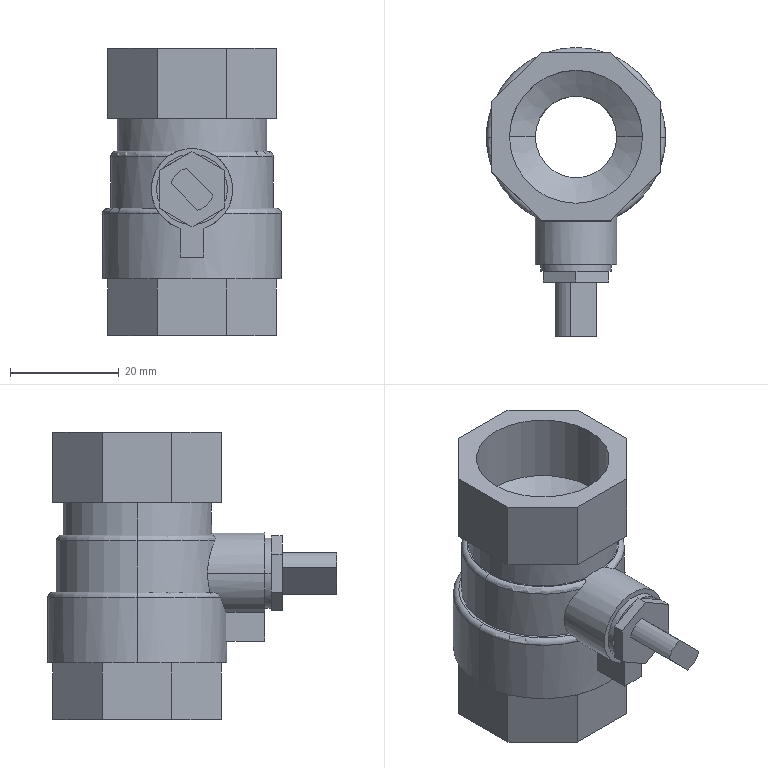Part | SolidWorks | features ICE 10, HoleWzd 2, 3DProfileFeature 1, Extrusion 1, Fillet 1 | 1 solid | 93 faces | box 33 x 53.25 x 53 mm | volume 25680 mm3 | plane 63 | cylinder 20 | torus 6 | cone 4 | commonest cylinder face diameters 15 x5 24.5 x4 30 x3 8 x2 13 x2 27.5 x2